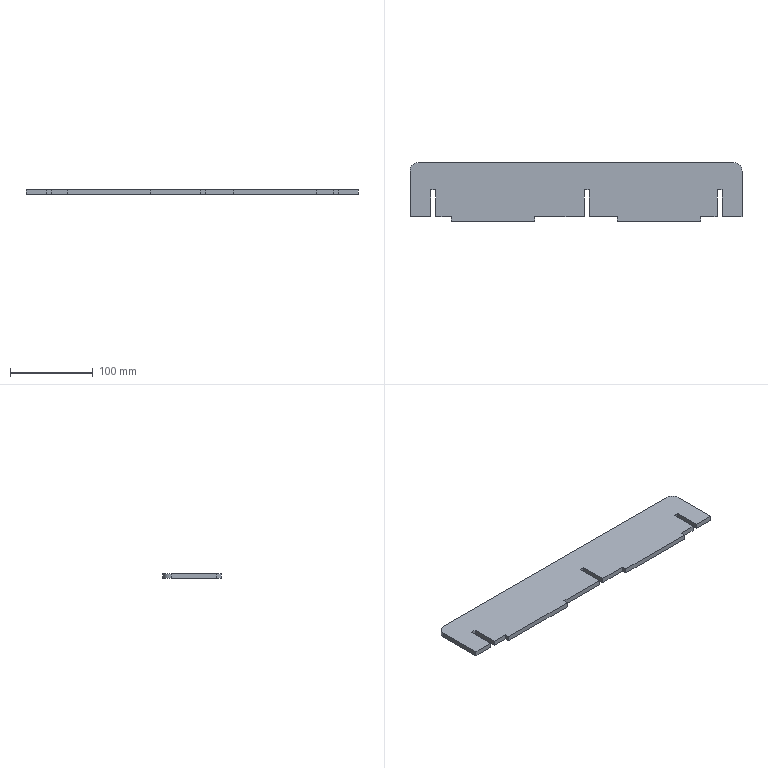Part | SolidWorks | features FlatPattern 1, SMBaseFlange 1, SheetMetal 1 | 1 solid | 28 faces | box 400 x 70.5 x 6 mm | volume 158832 mm3 | plane 26 | cylinder 2 | commonest cylinder face diameters 20 x2
STEP:
#1=CARTESIAN_POINT('',(117.03,-549.5,0.));
#2=VERTEX_POINT('',#1);
#3=CARTESIAN_POINT('',(117.03,-494.5,0.));
#4=VERTEX_POINT('',#3);
#5=CARTESIAN_POINT('',(117.03,-549.5,0.));
#6=DIRECTION('',(0.,1.,0.));
#7=VECTOR('',#6,1000.);
#8=LINE('',#5,#7);
#9=EDGE_CURVE('',#2,#4,#8,.T.);
#10=ORIENTED_EDGE('',*,*,#9,.F.);
#11=CARTESIAN_POINT('',(117.03,-549.5,-6.));
#12=VERTEX_POINT('',#11);
#13=CARTESIAN_POINT('',(117.03,-549.5,-6.));
#14=DIRECTION('',(0.,0.,1.));
#15=VECTOR('',#14,1000.);
#16=LINE('',#13,#15);
#17=EDGE_CURVE('',#12,#2,#16,.T.);
#18=ORIENTED_EDGE('',*,*,#17,.F.);
#19=CARTESIAN_POINT('',(117.03,-494.5,-6.));
#20=VERTEX_POINT('',#19);
#21=CARTESIAN_POINT('',(117.03,-549.5,-6.));
#22=DIRECTION('',(0.,1.,0.));
#23=VECTOR('',#22,1000.);
#24=LINE('',#21,#23);
#25=EDGE_CURVE('',#12,#20,#24,.T.);
#26=ORIENTED_EDGE('',*,*,#25,.T.);
#27=CARTESIAN_POINT('',(117.03,-494.5,-6.));
#28=DIRECTION('',(0.,0.,1.));
#29=VECTOR('',#28,1000.);
#30=LINE('',#27,#29);
#31=EDGE_CURVE('',#20,#4,#30,.T.);
#32=ORIENTED_EDGE('',*,*,#31,.T.);
#33=EDGE_LOOP('',(#10,#18,#26,#32));
#34=FACE_OUTER_BOUND('',#33,.T.);
#35=CARTESIAN_POINT('',(117.03,-549.5,-6.));
#36=DIRECTION('',(1.,0.,0.));
#37=DIRECTION('',(0.,0.,-1.));
#38=AXIS2_PLACEMENT_3D('',#35,#36,#37);
#39=PLANE('',#38);
#40=ADVANCED_FACE('',(#34),#39,.T.);
#41=CARTESIAN_POINT('',(93.03,-549.5,0.));
#42=VERTEX_POINT('',#41);
#43=CARTESIAN_POINT('',(117.03,-549.5,0.));
#44=DIRECTION('',(1.,0.,0.));
#45=VECTOR('',#44,1000.);
#46=LINE('',#43,#45);
#47=EDGE_CURVE('',#42,#2,#46,.T.);
#48=ORIENTED_EDGE('',*,*,#47,.F.);
#49=CARTESIAN_POINT('',(93.03,-549.5,-6.));
#50=VERTEX_POINT('',#49);
#51=CARTESIAN_POINT('',(93.03,-549.5,-6.));
#52=DIRECTION('',(0.,0.,1.));
#53=VECTOR('',#52,1000.);
#54=LINE('',#51,#53);
#55=EDGE_CURVE('',#50,#42,#54,.T.);
#56=ORIENTED_EDGE('',*,*,#55,.F.);
#57=CARTESIAN_POINT('',(117.03,-549.5,-6.));
#58=DIRECTION('',(1.,0.,0.));
#59=VECTOR('',#58,1000.);
#60=LINE('',#57,#59);
#61=EDGE_CURVE('',#50,#12,#60,.T.);
#62=ORIENTED_EDGE('',*,*,#61,.T.);
#63=ORIENTED_EDGE('',*,*,#17,.T.);
#64=EDGE_LOOP('',(#48,#56,#62,#63));
#65=FACE_OUTER_BOUND('',#64,.T.);
#66=CARTESIAN_POINT('',(117.03,-549.5,-6.));
#67=DIRECTION('',(0.,-1.,0.));
#68=DIRECTION('',(1.,0.,0.));
#69=AXIS2_PLACEMENT_3D('',#66,#67,#68);
#70=PLANE('',#69);
#71=ADVANCED_FACE('',(#65),#70,.T.);
#72=CARTESIAN_POINT('',(93.03,-517.,0.));
#73=VERTEX_POINT('',#72);
#74=CARTESIAN_POINT('',(93.03,-549.5,0.));
#75=DIRECTION('',(0.,-1.,0.));
#76=VECTOR('',#75,1000.);
#77=LINE('',#74,#76);
#78=EDGE_CURVE('',#73,#42,#77,.T.);
#79=ORIENTED_EDGE('',*,*,#78,.F.);
#80=CARTESIAN_POINT('',(93.03,-517.,-6.));
#81=VERTEX_POINT('',#80);
#82=CARTESIAN_POINT('',(93.03,-517.,-6.));
#83=DIRECTION('',(0.,0.,1.));
#84=VECTOR('',#83,1000.);
#85=LINE('',#82,#84);
#86=EDGE_CURVE('',#81,#73,#85,.T.);
#87=ORIENTED_EDGE('',*,*,#86,.F.);
#88=CARTESIAN_POINT('',(93.03,-549.5,-6.));
#89=DIRECTION('',(0.,-1.,0.));
#90=VECTOR('',#89,1000.);
#91=LINE('',#88,#90);
#92=EDGE_CURVE('',#81,#50,#91,.T.);
#93=ORIENTED_EDGE('',*,*,#92,.T.);
#94=ORIENTED_EDGE('',*,*,#55,.T.);
#95=EDGE_LOOP('',(#79,#87,#93,#94));
#96=FACE_OUTER_BOUND('',#95,.T.);
#97=CARTESIAN_POINT('',(93.03,-549.5,-6.));
#98=DIRECTION('',(-1.,0.,0.));
#99=DIRECTION('',(0.,-1.,0.));
#100=AXIS2_PLACEMENT_3D('',#97,#98,#99);
#101=PLANE('',#100);
#102=ADVANCED_FACE('',(#96),#101,.T.);
#103=CARTESIAN_POINT('',(87.03,-517.,0.));
#104=VERTEX_POINT('',#103);
#105=CARTESIAN_POINT('',(93.03,-517.,0.));
#106=DIRECTION('',(1.,0.,0.));
#107=VECTOR('',#106,1000.);
#108=LINE('',#105,#107);
#109=EDGE_CURVE('',#104,#73,#108,.T.);
#110=ORIENTED_EDGE('',*,*,#109,.F.);
#111=CARTESIAN_POINT('',(87.03,-517.,-6.));
#112=VERTEX_POINT('',#111);
#113=CARTESIAN_POINT('',(87.03,-517.,-6.));
#114=DIRECTION('',(0.,0.,1.));
#115=VECTOR('',#114,1000.);
#116=LINE('',#113,#115);
#117=EDGE_CURVE('',#112,#104,#116,.T.);
#118=ORIENTED_EDGE('',*,*,#117,.F.);
#119=CARTESIAN_POINT('',(93.03,-517.,-6.));
#120=DIRECTION('',(1.,0.,0.));
#121=VECTOR('',#120,1000.);
#122=LINE('',#119,#121);
#123=EDGE_CURVE('',#112,#81,#122,.T.);
#124=ORIENTED_EDGE('',*,*,#123,.T.);
#125=ORIENTED_EDGE('',*,*,#86,.T.);
#126=EDGE_LOOP('',(#110,#118,#124,#125));
#127=FACE_OUTER_BOUND('',#126,.T.);
#128=CARTESIAN_POINT('',(93.03,-517.,-6.));
#129=DIRECTION('',(0.,-1.,0.));
#130=DIRECTION('',(0.,0.,-1.));
#131=AXIS2_PLACEMENT_3D('',#128,#129,#130);
#132=PLANE('',#131);
#133=ADVANCED_FACE('',(#127),#132,.T.);
#134=CARTESIAN_POINT('',(87.03,-549.5,0.));
#135=VERTEX_POINT('',#134);
#136=CARTESIAN_POINT('',(87.03,-517.,0.));
#137=DIRECTION('',(0.,1.,0.));
#138=VECTOR('',#137,1000.);
#139=LINE('',#136,#138);
#140=EDGE_CURVE('',#135,#104,#139,.T.);
#141=ORIENTED_EDGE('',*,*,#140,.F.);
#142=CARTESIAN_POINT('',(87.03,-549.5,-6.));
#143=VERTEX_POINT('',#142);
#144=CARTESIAN_POINT('',(87.03,-549.5,-6.));
#145=DIRECTION('',(0.,0.,1.));
#146=VECTOR('',#145,1000.);
#147=LINE('',#144,#146);
#148=EDGE_CURVE('',#143,#135,#147,.T.);
#149=ORIENTED_EDGE('',*,*,#148,.F.);
#150=CARTESIAN_POINT('',(87.03,-517.,-6.));
#151=DIRECTION('',(0.,1.,0.));
#152=VECTOR('',#151,1000.);
#153=LINE('',#150,#152);
#154=EDGE_CURVE('',#143,#112,#153,.T.);
#155=ORIENTED_EDGE('',*,*,#154,.T.);
#156=ORIENTED_EDGE('',*,*,#117,.T.);
#157=EDGE_LOOP('',(#141,#149,#155,#156));
#158=FACE_OUTER_BOUND('',#157,.T.);
#159=CARTESIAN_POINT('',(87.03,-517.,-6.));
#160=DIRECTION('',(1.,0.,0.));
#161=DIRECTION('',(0.,0.,-1.));
#162=AXIS2_PLACEMENT_3D('',#159,#160,#161);
#163=PLANE('',#162);
#164=ADVANCED_FACE('',(#158),#163,.T.);
#165=CARTESIAN_POINT('',(67.03,-549.5,0.));
#166=VERTEX_POINT('',#165);
#167=CARTESIAN_POINT('',(87.03,-549.5,0.));
#168=DIRECTION('',(1.,0.,0.));
#169=VECTOR('',#168,1000.);
#170=LINE('',#167,#169);
#171=EDGE_CURVE('',#166,#135,#170,.T.);
#172=ORIENTED_EDGE('',*,*,#171,.F.);
#173=CARTESIAN_POINT('',(67.03,-549.5,-6.));
#174=VERTEX_POINT('',#173);
#175=CARTESIAN_POINT('',(67.03,-549.5,-6.));
#176=DIRECTION('',(0.,0.,1.));
#177=VECTOR('',#176,1000.);
#178=LINE('',#175,#177);
#179=EDGE_CURVE('',#174,#166,#178,.T.);
#180=ORIENTED_EDGE('',*,*,#179,.F.);
#181=CARTESIAN_POINT('',(87.03,-549.5,-6.));
#182=DIRECTION('',(1.,0.,0.));
#183=VECTOR('',#182,1000.);
#184=LINE('',#181,#183);
#185=EDGE_CURVE('',#174,#143,#184,.T.);
#186=ORIENTED_EDGE('',*,*,#185,.T.);
#187=ORIENTED_EDGE('',*,*,#148,.T.);
#188=EDGE_LOOP('',(#172,#180,#186,#187));
#189=FACE_OUTER_BOUND('',#188,.T.);
#190=CARTESIAN_POINT('',(87.03,-549.5,-6.));
#191=DIRECTION('',(0.,-1.,0.));
#192=DIRECTION('',(1.,0.,0.));
#193=AXIS2_PLACEMENT_3D('',#190,#191,#192);
#194=PLANE('',#193);
#195=ADVANCED_FACE('',(#189),#194,.T.);
#196=CARTESIAN_POINT('',(67.03,-555.,0.));
#197=VERTEX_POINT('',#196);
#198=CARTESIAN_POINT('',(67.03,-549.5,0.));
#199=DIRECTION('',(0.,1.,0.));
#200=VECTOR('',#199,1000.);
#201=LINE('',#198,#200);
#202=EDGE_CURVE('',#197,#166,#201,.T.);
#203=ORIENTED_EDGE('',*,*,#202,.F.);
#204=CARTESIAN_POINT('',(67.03,-555.,-6.));
#205=VERTEX_POINT('',#204);
#206=CARTESIAN_POINT('',(67.03,-555.,-6.));
#207=DIRECTION('',(0.,0.,1.));
#208=VECTOR('',#207,1000.);
#209=LINE('',#206,#208);
#210=EDGE_CURVE('',#205,#197,#209,.T.);
#211=ORIENTED_EDGE('',*,*,#210,.F.);
#212=CARTESIAN_POINT('',(67.03,-549.5,-6.));
#213=DIRECTION('',(0.,1.,0.));
#214=VECTOR('',#213,1000.);
#215=LINE('',#212,#214);
#216=EDGE_CURVE('',#205,#174,#215,.T.);
#217=ORIENTED_EDGE('',*,*,#216,.T.);
#218=ORIENTED_EDGE('',*,*,#179,.T.);
#219=EDGE_LOOP('',(#203,#211,#217,#218));
#220=FACE_OUTER_BOUND('',#219,.T.);
#221=CARTESIAN_POINT('',(67.03,-549.5,-6.));
#222=DIRECTION('',(1.,0.,0.));
#223=DIRECTION('',(0.,0.,-1.));
#224=AXIS2_PLACEMENT_3D('',#221,#222,#223);
#225=PLANE('',#224);
#226=ADVANCED_FACE('',(#220),#225,.T.);
#227=CARTESIAN_POINT('',(-32.97,-555.,0.));
#228=VERTEX_POINT('',#227);
#229=CARTESIAN_POINT('',(67.03,-555.,0.));
#230=DIRECTION('',(1.,0.,0.));
#231=VECTOR('',#230,1000.);
#232=LINE('',#229,#231);
#233=EDGE_CURVE('',#228,#197,#232,.T.);
#234=ORIENTED_EDGE('',*,*,#233,.F.);
#235=CARTESIAN_POINT('',(-32.97,-555.,-6.));
#236=VERTEX_POINT('',#235);
#237=CARTESIAN_POINT('',(-32.97,-555.,-6.));
#238=DIRECTION('',(0.,0.,1.));
#239=VECTOR('',#238,1000.);
#240=LINE('',#237,#239);
#241=EDGE_CURVE('',#236,#228,#240,.T.);
#242=ORIENTED_EDGE('',*,*,#241,.F.);
#243=CARTESIAN_POINT('',(67.03,-555.,-6.));
#244=DIRECTION('',(1.,0.,0.));
#245=VECTOR('',#244,1000.);
#246=LINE('',#243,#245);
#247=EDGE_CURVE('',#236,#205,#246,.T.);
#248=ORIENTED_EDGE('',*,*,#247,.T.);
#249=ORIENTED_EDGE('',*,*,#210,.T.);
#250=EDGE_LOOP('',(#234,#242,#248,#249));
#251=FACE_OUTER_BOUND('',#250,.T.);
#252=CARTESIAN_POINT('',(67.03,-555.,-6.));
#253=DIRECTION('',(0.,-1.,0.));
#254=DIRECTION('',(0.,0.,-1.));
#255=AXIS2_PLACEMENT_3D('',#252,#253,#254);
#256=PLANE('',#255);
#257=ADVANCED_FACE('',(#251),#256,.T.);
#258=CARTESIAN_POINT('',(-32.97,-549.5,0.));
#259=VERTEX_POINT('',#258);
#260=CARTESIAN_POINT('',(-32.97,-555.,0.));
#261=DIRECTION('',(0.,-1.,0.));
#262=VECTOR('',#261,1000.);
#263=LINE('',#260,#262);
#264=EDGE_CURVE('',#259,#228,#263,.T.);
#265=ORIENTED_EDGE('',*,*,#264,.F.);
#266=CARTESIAN_POINT('',(-32.97,-549.5,-6.));
#267=VERTEX_POINT('',#266);
#268=CARTESIAN_POINT('',(-32.97,-549.5,-6.));
#269=DIRECTION('',(0.,0.,1.));
#270=VECTOR('',#269,1000.);
#271=LINE('',#268,#270);
#272=EDGE_CURVE('',#267,#259,#271,.T.);
#273=ORIENTED_EDGE('',*,*,#272,.F.);
#274=CARTESIAN_POINT('',(-32.97,-555.,-6.));
#275=DIRECTION('',(0.,-1.,0.));
#276=VECTOR('',#275,1000.);
#277=LINE('',#274,#276);
#278=EDGE_CURVE('',#267,#236,#277,.T.);
#279=ORIENTED_EDGE('',*,*,#278,.T.);
#280=ORIENTED_EDGE('',*,*,#241,.T.);
#281=EDGE_LOOP('',(#265,#273,#279,#280));
#282=FACE_OUTER_BOUND('',#281,.T.);
#283=CARTESIAN_POINT('',(-32.97,-555.,-6.));
#284=DIRECTION('',(-1.,0.,0.));
#285=DIRECTION('',(0.,0.,1.));
#286=AXIS2_PLACEMENT_3D('',#283,#284,#285);
#287=PLANE('',#286);
#288=ADVANCED_FACE('',(#282),#287,.T.);
#289=CARTESIAN_POINT('',(-66.97,-549.5,0.));
#290=VERTEX_POINT('',#289);
#291=CARTESIAN_POINT('',(-32.97,-549.5,0.));
#292=DIRECTION('',(1.,0.,0.));
#293=VECTOR('',#292,1000.);
#294=LINE('',#291,#293);
#295=EDGE_CURVE('',#290,#259,#294,.T.);
#296=ORIENTED_EDGE('',*,*,#295,.F.);
#297=CARTESIAN_POINT('',(-66.97,-549.5,-6.));
#298=VERTEX_POINT('',#297);
#299=CARTESIAN_POINT('',(-66.97,-549.5,-6.));
#300=DIRECTION('',(0.,0.,1.));
#301=VECTOR('',#300,1000.);
#302=LINE('',#299,#301);
#303=EDGE_CURVE('',#298,#290,#302,.T.);
#304=ORIENTED_EDGE('',*,*,#303,.F.);
#305=CARTESIAN_POINT('',(-32.97,-549.5,-6.));
#306=DIRECTION('',(1.,0.,0.));
#307=VECTOR('',#306,1000.);
#308=LINE('',#305,#307);
#309=EDGE_CURVE('',#298,#267,#308,.T.);
#310=ORIENTED_EDGE('',*,*,#309,.T.);
#311=ORIENTED_EDGE('',*,*,#272,.T.);
#312=EDGE_LOOP('',(#296,#304,#310,#311));
#313=FACE_OUTER_BOUND('',#312,.T.);
#314=CARTESIAN_POINT('',(-32.97,-549.5,-6.));
#315=DIRECTION('',(0.,-1.,0.));
#316=DIRECTION('',(1.,0.,0.));
#317=AXIS2_PLACEMENT_3D('',#314,#315,#316);
#318=PLANE('',#317);
#319=ADVANCED_FACE('',(#313),#318,.T.);
#320=CARTESIAN_POINT('',(-66.97,-517.,0.));
#321=VERTEX_POINT('',#320);
#322=CARTESIAN_POINT('',(-66.97,-549.5,0.));
#323=DIRECTION('',(0.,-1.,0.));
#324=VECTOR('',#323,1000.);
#325=LINE('',#322,#324);
#326=EDGE_CURVE('',#321,#290,#325,.T.);
#327=ORIENTED_EDGE('',*,*,#326,.F.);
#328=CARTESIAN_POINT('',(-66.97,-517.,-6.));
#329=VERTEX_POINT('',#328);
#330=CARTESIAN_POINT('',(-66.97,-517.,-6.));
#331=DIRECTION('',(0.,0.,1.));
#332=VECTOR('',#331,1000.);
#333=LINE('',#330,#332);
#334=EDGE_CURVE('',#329,#321,#333,.T.);
#335=ORIENTED_EDGE('',*,*,#334,.F.);
#336=CARTESIAN_POINT('',(-66.97,-549.5,-6.));
#337=DIRECTION('',(0.,-1.,0.));
#338=VECTOR('',#337,1000.);
#339=LINE('',#336,#338);
#340=EDGE_CURVE('',#329,#298,#339,.T.);
#341=ORIENTED_EDGE('',*,*,#340,.T.);
#342=ORIENTED_EDGE('',*,*,#303,.T.);
#343=EDGE_LOOP('',(#327,#335,#341,#342));
#344=FACE_OUTER_BOUND('',#343,.T.);
#345=CARTESIAN_POINT('',(-66.97,-549.5,-6.));
#346=DIRECTION('',(-1.,0.,0.));
#347=DIRECTION('',(0.,0.,1.));
#348=AXIS2_PLACEMENT_3D('',#345,#346,#347);
#349=PLANE('',#348);
#350=ADVANCED_FACE('',(#344),#349,.T.);
#351=CARTESIAN_POINT('',(-72.97,-517.,0.));
#352=VERTEX_POINT('',#351);
#353=CARTESIAN_POINT('',(-66.97,-517.,0.));
#354=DIRECTION('',(1.,0.,0.));
#355=VECTOR('',#354,1000.);
#356=LINE('',#353,#355);
#357=EDGE_CURVE('',#352,#321,#356,.T.);
#358=ORIENTED_EDGE('',*,*,#357,.F.);
#359=CARTESIAN_POINT('',(-72.97,-517.,-6.));
#360=VERTEX_POINT('',#359);
#361=CARTESIAN_POINT('',(-72.97,-517.,-6.));
#362=DIRECTION('',(0.,0.,1.));
#363=VECTOR('',#362,1000.);
#364=LINE('',#361,#363);
#365=EDGE_CURVE('',#360,#352,#364,.T.);
#366=ORIENTED_EDGE('',*,*,#365,.F.);
#367=CARTESIAN_POINT('',(-66.97,-517.,-6.));
#368=DIRECTION('',(1.,0.,0.));
#369=VECTOR('',#368,1000.);
#370=LINE('',#367,#369);
#371=EDGE_CURVE('',#360,#329,#370,.T.);
#372=ORIENTED_EDGE('',*,*,#371,.T.);
#373=ORIENTED_EDGE('',*,*,#334,.T.);
#374=EDGE_LOOP('',(#358,#366,#372,#373));
#375=FACE_OUTER_BOUND('',#374,.T.);
#376=CARTESIAN_POINT('',(-66.97,-517.,-6.));
#377=DIRECTION('',(0.,-1.,0.));
#378=DIRECTION('',(0.,0.,-1.));
#379=AXIS2_PLACEMENT_3D('',#376,#377,#378);
#380=PLANE('',#379);
#381=ADVANCED_FACE('',(#375),#380,.T.);
#382=CARTESIAN_POINT('',(-72.97,-549.5,0.));
#383=VERTEX_POINT('',#382);
#384=CARTESIAN_POINT('',(-72.97,-517.,0.));
#385=DIRECTION('',(0.,1.,0.));
#386=VECTOR('',#385,1000.);
#387=LINE('',#384,#386);
#388=EDGE_CURVE('',#383,#352,#387,.T.);
#389=ORIENTED_EDGE('',*,*,#388,.F.);
#390=CARTESIAN_POINT('',(-72.97,-549.5,-6.));
#391=VERTEX_POINT('',#390);
#392=CARTESIAN_POINT('',(-72.97,-549.5,-6.));
#393=DIRECTION('',(0.,0.,1.));
#394=VECTOR('',#393,1000.);
#395=LINE('',#392,#394);
#396=EDGE_CURVE('',#391,#383,#395,.T.);
#397=ORIENTED_EDGE('',*,*,#396,.F.);
#398=CARTESIAN_POINT('',(-72.97,-517.,-6.));
#399=DIRECTION('',(0.,1.,0.));
#400=VECTOR('',#399,1000.);
#401=LINE('',#398,#400);
#402=EDGE_CURVE('',#391,#360,#401,.T.);
#403=ORIENTED_EDGE('',*,*,#402,.T.);
#404=ORIENTED_EDGE('',*,*,#365,.T.);
#405=EDGE_LOOP('',(#389,#397,#403,#404));
#406=FACE_OUTER_BOUND('',#405,.T.);
#407=CARTESIAN_POINT('',(-72.97,-517.,-6.));
#408=DIRECTION('',(1.,0.,0.));
#409=DIRECTION('',(0.,0.,-1.));
#410=AXIS2_PLACEMENT_3D('',#407,#408,#409);
#411=PLANE('',#410);
#412=ADVANCED_FACE('',(#406),#411,.T.);
#413=CARTESIAN_POINT('',(-132.97,-549.5,0.));
#414=VERTEX_POINT('',#413);
#415=CARTESIAN_POINT('',(-72.97,-549.5,0.));
#416=DIRECTION('',(1.,0.,0.));
#417=VECTOR('',#416,1000.);
#418=LINE('',#415,#417);
#419=EDGE_CURVE('',#414,#383,#418,.T.);
#420=ORIENTED_EDGE('',*,*,#419,.F.);
#421=CARTESIAN_POINT('',(-132.97,-549.5,-6.));
#422=VERTEX_POINT('',#421);
#423=CARTESIAN_POINT('',(-132.97,-549.5,-6.));
#424=DIRECTION('',(0.,0.,1.));
#425=VECTOR('',#424,1000.);
#426=LINE('',#423,#425);
#427=EDGE_CURVE('',#422,#414,#426,.T.);
#428=ORIENTED_EDGE('',*,*,#427,.F.);
#429=CARTESIAN_POINT('',(-72.97,-549.5,-6.));
#430=DIRECTION('',(1.,0.,0.));
#431=VECTOR('',#430,1000.);
#432=LINE('',#429,#431);
#433=EDGE_CURVE('',#422,#391,#432,.T.);
#434=ORIENTED_EDGE('',*,*,#433,.T.);
#435=ORIENTED_EDGE('',*,*,#396,.T.);
#436=EDGE_LOOP('',(#420,#428,#434,#435));
#437=FACE_OUTER_BOUND('',#436,.T.);
#438=CARTESIAN_POINT('',(-72.97,-549.5,-6.));
#439=DIRECTION('',(0.,-1.,0.));
#440=DIRECTION('',(1.,0.,0.));
#441=AXIS2_PLACEMENT_3D('',#438,#439,#440);
#442=PLANE('',#441);
#443=ADVANCED_FACE('',(#437),#442,.T.);
#444=CARTESIAN_POINT('',(-132.97,-555.,0.));
#445=VERTEX_POINT('',#444);
#446=CARTESIAN_POINT('',(-132.97,-555.,0.));
#447=DIRECTION('',(0.,1.,0.));
#448=VECTOR('',#447,1000.);
#449=LINE('',#446,#448);
#450=EDGE_CURVE('',#445,#414,#449,.T.);
#451=ORIENTED_EDGE('',*,*,#450,.F.);
#452=CARTESIAN_POINT('',(-132.97,-555.,-6.));
#453=VERTEX_POINT('',#452);
#454=CARTESIAN_POINT('',(-132.97,-555.,-6.));
#455=DIRECTION('',(0.,0.,1.));
#456=VECTOR('',#455,1000.);
#457=LINE('',#454,#456);
#458=EDGE_CURVE('',#453,#445,#457,.T.);
#459=ORIENTED_EDGE('',*,*,#458,.F.);
#460=CARTESIAN_POINT('',(-132.97,-555.,-6.));
#461=DIRECTION('',(0.,1.,0.));
#462=VECTOR('',#461,1000.);
#463=LINE('',#460,#462);
#464=EDGE_CURVE('',#453,#422,#463,.T.);
#465=ORIENTED_EDGE('',*,*,#464,.T.);
#466=ORIENTED_EDGE('',*,*,#427,.T.);
#467=EDGE_LOOP('',(#451,#459,#465,#466));
#468=FACE_OUTER_BOUND('',#467,.T.);
#469=CARTESIAN_POINT('',(-132.97,-555.,-6.));
#470=DIRECTION('',(1.,0.,0.));
#471=DIRECTION('',(0.,0.,-1.));
#472=AXIS2_PLACEMENT_3D('',#469,#470,#471);
#473=PLANE('',#472);
#474=ADVANCED_FACE('',(#468),#473,.T.);
#475=CARTESIAN_POINT('',(-232.97,-555.,0.));
#476=VERTEX_POINT('',#475);
#477=CARTESIAN_POINT('',(-232.97,-555.,0.));
#478=DIRECTION('',(1.,0.,0.));
#479=VECTOR('',#478,1000.);
#480=LINE('',#477,#479);
#481=EDGE_CURVE('',#476,#445,#480,.T.);
#482=ORIENTED_EDGE('',*,*,#481,.F.);
#483=CARTESIAN_POINT('',(-232.97,-555.,-6.));
#484=VERTEX_POINT('',#483);
#485=CARTESIAN_POINT('',(-232.97,-555.,-6.));
#486=DIRECTION('',(0.,0.,1.));
#487=VECTOR('',#486,1000.);
#488=LINE('',#485,#487);
#489=EDGE_CURVE('',#484,#476,#488,.T.);
#490=ORIENTED_EDGE('',*,*,#489,.F.);
#491=CARTESIAN_POINT('',(-232.97,-555.,-6.));
#492=DIRECTION('',(1.,0.,0.));
#493=VECTOR('',#492,1000.);
#494=LINE('',#491,#493);
#495=EDGE_CURVE('',#484,#453,#494,.T.);
#496=ORIENTED_EDGE('',*,*,#495,.T.);
#497=ORIENTED_EDGE('',*,*,#458,.T.);
#498=EDGE_LOOP('',(#482,#490,#496,#497));
#499=FACE_OUTER_BOUND('',#498,.T.);
#500=CARTESIAN_POINT('',(-232.97,-555.,-6.));
#501=DIRECTION('',(0.,-1.,0.));
#502=DIRECTION('',(0.,0.,-1.));
#503=AXIS2_PLACEMENT_3D('',#500,#501,#502);
#504=PLANE('',#503);
#505=ADVANCED_FACE('',(#499),#504,.T.);
#506=CARTESIAN_POINT('',(-232.97,-549.5,0.));
#507=VERTEX_POINT('',#506);
#508=CARTESIAN_POINT('',(-232.97,-549.5,0.));
#509=DIRECTION('',(0.,-1.,0.));
#510=VECTOR('',#509,1000.);
#511=LINE('',#508,#510);
#512=EDGE_CURVE('',#507,#476,#511,.T.);
#513=ORIENTED_EDGE('',*,*,#512,.F.);
#514=CARTESIAN_POINT('',(-232.97,-549.5,-6.));
#515=VERTEX_POINT('',#514);
#516=CARTESIAN_POINT('',(-232.97,-549.5,-6.));
#517=DIRECTION('',(0.,0.,1.));
#518=VECTOR('',#517,1000.);
#519=LINE('',#516,#518);
#520=EDGE_CURVE('',#515,#507,#519,.T.);
#521=ORIENTED_EDGE('',*,*,#520,.F.);
#522=CARTESIAN_POINT('',(-232.97,-549.5,-6.));
#523=DIRECTION('',(0.,-1.,0.));
#524=VECTOR('',#523,1000.);
#525=LINE('',#522,#524);
#526=EDGE_CURVE('',#515,#484,#525,.T.);
#527=ORIENTED_EDGE('',*,*,#526,.T.);
#528=ORIENTED_EDGE('',*,*,#489,.T.);
#529=EDGE_LOOP('',(#513,#521,#527,#528));
#530=FACE_OUTER_BOUND('',#529,.T.);
#531=CARTESIAN_POINT('',(-232.97,-549.5,-6.));
#532=DIRECTION('',(-1.,0.,0.));
#533=DIRECTION('',(0.,0.,1.));
#534=AXIS2_PLACEMENT_3D('',#531,#532,#533);
#535=PLANE('',#534);
#536=ADVANCED_FACE('',(#530),#535,.T.);
#537=CARTESIAN_POINT('',(-251.97,-549.5,0.));
#538=VERTEX_POINT('',#537);
#539=CARTESIAN_POINT('',(-232.97,-549.5,0.));
#540=DIRECTION('',(1.,0.,0.));
#541=VECTOR('',#540,1000.);
#542=LINE('',#539,#541);
#543=EDGE_CURVE('',#538,#507,#542,.T.);
#544=ORIENTED_EDGE('',*,*,#543,.F.);
#545=CARTESIAN_POINT('',(-251.97,-549.5,-6.));
#546=VERTEX_POINT('',#545);
#547=CARTESIAN_POINT('',(-251.97,-549.5,-6.));
#548=DIRECTION('',(0.,0.,1.));
#549=VECTOR('',#548,1000.);
#550=LINE('',#547,#549);
#551=EDGE_CURVE('',#546,#538,#550,.T.);
#552=ORIENTED_EDGE('',*,*,#551,.F.);
#553=CARTESIAN_POINT('',(-232.97,-549.5,-6.));
#554=DIRECTION('',(1.,0.,0.));
#555=VECTOR('',#554,1000.);
#556=LINE('',#553,#555);
#557=EDGE_CURVE('',#546,#515,#556,.T.);
#558=ORIENTED_EDGE('',*,*,#557,.T.);
#559=ORIENTED_EDGE('',*,*,#520,.T.);
#560=EDGE_LOOP('',(#544,#552,#558,#559));
#561=FACE_OUTER_BOUND('',#560,.T.);
#562=CARTESIAN_POINT('',(-232.97,-549.5,-6.));
#563=DIRECTION('',(0.,-1.,0.));
#564=DIRECTION('',(1.,0.,0.));
#565=AXIS2_PLACEMENT_3D('',#562,#563,#564);
#566=PLANE('',#565);
#567=ADVANCED_FACE('',(#561),#566,.T.);
#568=CARTESIAN_POINT('',(-251.97,-517.,0.));
#569=VERTEX_POINT('',#568);
#570=CARTESIAN_POINT('',(-251.97,-549.5,0.));
#571=DIRECTION('',(0.,-1.,0.));
#572=VECTOR('',#571,1000.);
#573=LINE('',#570,#572);
#574=EDGE_CURVE('',#569,#538,#573,.T.);
#575=ORIENTED_EDGE('',*,*,#574,.F.);
#576=CARTESIAN_POINT('',(-251.97,-517.,-6.));
#577=VERTEX_POINT('',#576);
#578=CARTESIAN_POINT('',(-251.97,-517.,-6.));
#579=DIRECTION('',(0.,0.,1.));
#580=VECTOR('',#579,1000.);
#581=LINE('',#578,#580);
#582=EDGE_CURVE('',#577,#569,#581,.T.);
#583=ORIENTED_EDGE('',*,*,#582,.F.);
#584=CARTESIAN_POINT('',(-251.97,-549.5,-6.));
#585=DIRECTION('',(0.,-1.,0.));
#586=VECTOR('',#585,1000.);
#587=LINE('',#584,#586);
#588=EDGE_CURVE('',#577,#546,#587,.T.);
#589=ORIENTED_EDGE('',*,*,#588,.T.);
#590=ORIENTED_EDGE('',*,*,#551,.T.);
#591=EDGE_LOOP('',(#575,#583,#589,#590));
#592=FACE_OUTER_BOUND('',#591,.T.);
#593=CARTESIAN_POINT('',(-251.97,-549.5,-6.));
#594=DIRECTION('',(-1.,0.,0.));
#595=DIRECTION('',(0.,-1.,0.));
#596=AXIS2_PLACEMENT_3D('',#593,#594,#595);
#597=PLANE('',#596);
#598=ADVANCED_FACE('',(#592),#597,.T.);
#599=CARTESIAN_POINT('',(-257.97,-517.,0.));
#600=VERTEX_POINT('',#599);
#601=CARTESIAN_POINT('',(-251.97,-517.,0.));
#602=DIRECTION('',(1.,0.,0.));
#603=VECTOR('',#602,1000.);
#604=LINE('',#601,#603);
#605=EDGE_CURVE('',#600,#569,#604,.T.);
#606=ORIENTED_EDGE('',*,*,#605,.F.);
#607=CARTESIAN_POINT('',(-257.97,-517.,-6.));
#608=VERTEX_POINT('',#607);
#609=CARTESIAN_POINT('',(-257.97,-517.,-6.));
#610=DIRECTION('',(0.,0.,1.));
#611=VECTOR('',#610,1000.);
#612=LINE('',#609,#611);
#613=EDGE_CURVE('',#608,#600,#612,.T.);
#614=ORIENTED_EDGE('',*,*,#613,.F.);
#615=CARTESIAN_POINT('',(-251.97,-517.,-6.));
#616=DIRECTION('',(1.,0.,0.));
#617=VECTOR('',#616,1000.);
#618=LINE('',#615,#617);
#619=EDGE_CURVE('',#608,#577,#618,.T.);
#620=ORIENTED_EDGE('',*,*,#619,.T.);
#621=ORIENTED_EDGE('',*,*,#582,.T.);
#622=EDGE_LOOP('',(#606,#614,#620,#621));
#623=FACE_OUTER_BOUND('',#622,.T.);
#624=CARTESIAN_POINT('',(-251.97,-517.,-6.));
#625=DIRECTION('',(0.,-1.,0.));
#626=DIRECTION('',(0.,0.,-1.));
#627=AXIS2_PLACEMENT_3D('',#624,#625,#626);
#628=PLANE('',#627);
#629=ADVANCED_FACE('',(#623),#628,.T.);
#630=CARTESIAN_POINT('',(-257.97,-549.5,0.));
#631=VERTEX_POINT('',#630);
#632=CARTESIAN_POINT('',(-257.97,-517.,0.));
#633=DIRECTION('',(0.,1.,0.));
#634=VECTOR('',#633,1000.);
#635=LINE('',#632,#634);
#636=EDGE_CURVE('',#631,#600,#635,.T.);
#637=ORIENTED_EDGE('',*,*,#636,.F.);
#638=CARTESIAN_POINT('',(-257.97,-549.5,-6.));
#639=VERTEX_POINT('',#638);
#640=CARTESIAN_POINT('',(-257.97,-549.5,-6.));
#641=DIRECTION('',(0.,0.,1.));
#642=VECTOR('',#641,1000.);
#643=LINE('',#640,#642);
#644=EDGE_CURVE('',#639,#631,#643,.T.);
#645=ORIENTED_EDGE('',*,*,#644,.F.);
#646=CARTESIAN_POINT('',(-257.97,-517.,-6.));
#647=DIRECTION('',(0.,1.,0.));
#648=VECTOR('',#647,1000.);
#649=LINE('',#646,#648);
#650=EDGE_CURVE('',#639,#608,#649,.T.);
#651=ORIENTED_EDGE('',*,*,#650,.T.);
#652=ORIENTED_EDGE('',*,*,#613,.T.);
#653=EDGE_LOOP('',(#637,#645,#651,#652));
#654=FACE_OUTER_BOUND('',#653,.T.);
#655=CARTESIAN_POINT('',(-257.97,-517.,-6.));
#656=DIRECTION('',(1.,0.,0.));
#657=DIRECTION('',(0.,0.,-1.));
#658=AXIS2_PLACEMENT_3D('',#655,#656,#657);
#659=PLANE('',#658);
#660=ADVANCED_FACE('',(#654),#659,.T.);
#661=CARTESIAN_POINT('',(-282.97,-549.5,0.));
#662=VERTEX_POINT('',#661);
#663=CARTESIAN_POINT('',(-257.97,-549.5,0.));
#664=DIRECTION('',(1.,0.,0.));
#665=VECTOR('',#664,1000.);
#666=LINE('',#663,#665);
#667=EDGE_CURVE('',#662,#631,#666,.T.);
#668=ORIENTED_EDGE('',*,*,#667,.F.);
#669=CARTESIAN_POINT('',(-282.97,-549.5,-6.));
#670=VERTEX_POINT('',#669);
#671=CARTESIAN_POINT('',(-282.97,-549.5,-6.));
#672=DIRECTION('',(0.,0.,1.));
#673=VECTOR('',#672,1000.);
#674=LINE('',#671,#673);
#675=EDGE_CURVE('',#670,#662,#674,.T.);
#676=ORIENTED_EDGE('',*,*,#675,.F.);
#677=CARTESIAN_POINT('',(-257.97,-549.5,-6.));
#678=DIRECTION('',(1.,0.,0.));
#679=VECTOR('',#678,1000.);
#680=LINE('',#677,#679);
#681=EDGE_CURVE('',#670,#639,#680,.T.);
#682=ORIENTED_EDGE('',*,*,#681,.T.);
#683=ORIENTED_EDGE('',*,*,#644,.T.);
#684=EDGE_LOOP('',(#668,#676,#682,#683));
#685=FACE_OUTER_BOUND('',#684,.T.);
#686=CARTESIAN_POINT('',(-257.97,-549.5,-6.));
#687=DIRECTION('',(0.,-1.,0.));
#688=DIRECTION('',(1.,0.,0.));
#689=AXIS2_PLACEMENT_3D('',#686,#687,#688);
#690=PLANE('',#689);
#691=ADVANCED_FACE('',(#685),#690,.T.);
#692=CARTESIAN_POINT('',(-282.97,-494.5,0.));
#693=VERTEX_POINT('',#692);
#694=CARTESIAN_POINT('',(-282.97,-549.5,0.));
#695=DIRECTION('',(0.,-1.,0.));
#696=VECTOR('',#695,1000.);
#697=LINE('',#694,#696);
#698=EDGE_CURVE('',#693,#662,#697,.T.);
#699=ORIENTED_EDGE('',*,*,#698,.F.);
#700=CARTESIAN_POINT('',(-282.97,-494.5,-6.));
#701=VERTEX_POINT('',#700);
#702=CARTESIAN_POINT('',(-282.97,-494.5,-6.));
#703=DIRECTION('',(0.,0.,1.));
#704=VECTOR('',#703,1000.);
#705=LINE('',#702,#704);
#706=EDGE_CURVE('',#701,#693,#705,.T.);
#707=ORIENTED_EDGE('',*,*,#706,.F.);
#708=CARTESIAN_POINT('',(-282.97,-549.5,-6.));
#709=DIRECTION('',(0.,-1.,0.));
#710=VECTOR('',#709,1000.);
#711=LINE('',#708,#710);
#712=EDGE_CURVE('',#701,#670,#711,.T.);
#713=ORIENTED_EDGE('',*,*,#712,.T.);
#714=ORIENTED_EDGE('',*,*,#675,.T.);
#715=EDGE_LOOP('',(#699,#707,#713,#714));
#716=FACE_OUTER_BOUND('',#715,.T.);
#717=CARTESIAN_POINT('',(-282.97,-549.5,-6.));
#718=DIRECTION('',(-1.,0.,0.));
#719=DIRECTION('',(0.,-1.,0.));
#720=AXIS2_PLACEMENT_3D('',#717,#718,#719);
#721=PLANE('',#720);
#722=ADVANCED_FACE('',(#716),#721,.T.);
#723=CARTESIAN_POINT('',(-272.97,-484.5,0.));
#724=VERTEX_POINT('',#723);
#725=CARTESIAN_POINT('',(-272.97,-494.5,0.));
#726=DIRECTION('',(0.,0.,1.));
#727=DIRECTION('',(1.,0.,0.));
#728=AXIS2_PLACEMENT_3D('',#725,#726,#727);
#729=CIRCLE('',#728,10.);
#730=EDGE_CURVE('',#724,#693,#729,.T.);
#731=ORIENTED_EDGE('',*,*,#730,.F.);
#732=CARTESIAN_POINT('',(-272.97,-484.5,-6.));
#733=VERTEX_POINT('',#732);
#734=CARTESIAN_POINT('',(-272.97,-484.5,-6.));
#735=DIRECTION('',(0.,0.,1.));
#736=VECTOR('',#735,1000.);
#737=LINE('',#734,#736);
#738=EDGE_CURVE('',#733,#724,#737,.T.);
#739=ORIENTED_EDGE('',*,*,#738,.F.);
#740=CARTESIAN_POINT('',(-272.97,-494.5,-6.));
#741=DIRECTION('',(0.,0.,1.));
#742=DIRECTION('',(1.,0.,0.));
#743=AXIS2_PLACEMENT_3D('',#740,#741,#742);
#744=CIRCLE('',#743,10.);
#745=EDGE_CURVE('',#733,#701,#744,.T.);
#746=ORIENTED_EDGE('',*,*,#745,.T.);
#747=ORIENTED_EDGE('',*,*,#706,.T.);
#748=EDGE_LOOP('',(#731,#739,#746,#747));
#749=FACE_OUTER_BOUND('',#748,.T.);
#750=CARTESIAN_POINT('',(-272.97,-494.5,-6.));
#751=DIRECTION('',(0.,0.,1.));
#752=DIRECTION('',(1.,0.,0.));
#753=AXIS2_PLACEMENT_3D('',#750,#751,#752);
#754=CYLINDRICAL_SURFACE('',#753,10.);
#755=ADVANCED_FACE('',(#749),#754,.T.);
#756=CARTESIAN_POINT('',(107.03,-484.5,0.));
#757=VERTEX_POINT('',#756);
#758=CARTESIAN_POINT('',(107.03,-484.5,0.));
#759=DIRECTION('',(-1.,0.,0.));
#760=VECTOR('',#759,1000.);
#761=LINE('',#758,#760);
#762=EDGE_CURVE('',#757,#724,#761,.T.);
#763=ORIENTED_EDGE('',*,*,#762,.F.);
#764=CARTESIAN_POINT('',(107.03,-484.5,-6.));
#765=VERTEX_POINT('',#764);
#766=CARTESIAN_POINT('',(107.03,-484.5,-6.));
#767=DIRECTION('',(0.,0.,1.));
#768=VECTOR('',#767,1000.);
#769=LINE('',#766,#768);
#770=EDGE_CURVE('',#765,#757,#769,.T.);
#771=ORIENTED_EDGE('',*,*,#770,.F.);
#772=CARTESIAN_POINT('',(107.03,-484.5,-6.));
#773=DIRECTION('',(-1.,0.,0.));
#774=VECTOR('',#773,1000.);
#775=LINE('',#772,#774);
#776=EDGE_CURVE('',#765,#733,#775,.T.);
#777=ORIENTED_EDGE('',*,*,#776,.T.);
#778=ORIENTED_EDGE('',*,*,#738,.T.);
#779=EDGE_LOOP('',(#763,#771,#777,#778));
#780=FACE_OUTER_BOUND('',#779,.T.);
#781=CARTESIAN_POINT('',(107.03,-484.5,-6.));
#782=DIRECTION('',(0.,1.,0.));
#783=DIRECTION('',(-1.,0.,0.));
#784=AXIS2_PLACEMENT_3D('',#781,#782,#783);
#785=PLANE('',#784);
#786=ADVANCED_FACE('',(#780),#785,.T.);
#787=CARTESIAN_POINT('',(107.03,-494.5,0.));
#788=DIRECTION('',(0.,0.,1.));
#789=DIRECTION('',(1.,0.,0.));
#790=AXIS2_PLACEMENT_3D('',#787,#788,#789);
#791=CIRCLE('',#790,10.);
#792=EDGE_CURVE('',#4,#757,#791,.T.);
#793=ORIENTED_EDGE('',*,*,#792,.F.);
#794=ORIENTED_EDGE('',*,*,#31,.F.);
#795=CARTESIAN_POINT('',(107.03,-494.5,-6.));
#796=DIRECTION('',(0.,0.,1.));
#797=DIRECTION('',(1.,0.,0.));
#798=AXIS2_PLACEMENT_3D('',#795,#796,#797);
#799=CIRCLE('',#798,10.);
#800=EDGE_CURVE('',#20,#765,#799,.T.);
#801=ORIENTED_EDGE('',*,*,#800,.T.);
#802=ORIENTED_EDGE('',*,*,#770,.T.);
#803=EDGE_LOOP('',(#793,#794,#801,#802));
#804=FACE_OUTER_BOUND('',#803,.T.);
#805=CARTESIAN_POINT('',(107.03,-494.5,-6.));
#806=DIRECTION('',(0.,0.,1.));
#807=DIRECTION('',(1.,0.,0.));
#808=AXIS2_PLACEMENT_3D('',#805,#806,#807);
#809=CYLINDRICAL_SURFACE('',#808,10.);
#810=ADVANCED_FACE('',(#804),#809,.T.);
#811=ORIENTED_EDGE('',*,*,#25,.F.);
#812=ORIENTED_EDGE('',*,*,#61,.F.);
#813=ORIENTED_EDGE('',*,*,#92,.F.);
#814=ORIENTED_EDGE('',*,*,#123,.F.);
#815=ORIENTED_EDGE('',*,*,#154,.F.);
#816=ORIENTED_EDGE('',*,*,#185,.F.);
#817=ORIENTED_EDGE('',*,*,#216,.F.);
#818=ORIENTED_EDGE('',*,*,#247,.F.);
#819=ORIENTED_EDGE('',*,*,#278,.F.);
#820=ORIENTED_EDGE('',*,*,#309,.F.);
#821=ORIENTED_EDGE('',*,*,#340,.F.);
#822=ORIENTED_EDGE('',*,*,#371,.F.);
#823=ORIENTED_EDGE('',*,*,#402,.F.);
#824=ORIENTED_EDGE('',*,*,#433,.F.);
#825=ORIENTED_EDGE('',*,*,#464,.F.);
#826=ORIENTED_EDGE('',*,*,#495,.F.);
#827=ORIENTED_EDGE('',*,*,#526,.F.);
#828=ORIENTED_EDGE('',*,*,#557,.F.);
#829=ORIENTED_EDGE('',*,*,#588,.F.);
#830=ORIENTED_EDGE('',*,*,#619,.F.);
#831=ORIENTED_EDGE('',*,*,#650,.F.);
#832=ORIENTED_EDGE('',*,*,#681,.F.);
#833=ORIENTED_EDGE('',*,*,#712,.F.);
#834=ORIENTED_EDGE('',*,*,#745,.F.);
#835=ORIENTED_EDGE('',*,*,#776,.F.);
#836=ORIENTED_EDGE('',*,*,#800,.F.);
#837=EDGE_LOOP('',(#811,#812,#813,#814,#815,#816,#817,#818,#819,#820,#821,#822,#823,#824,#825,#826,#827,#828,#829,#830,#831,#832,#833,#834,#835,#836));
#838=FACE_OUTER_BOUND('',#837,.T.);
#839=CARTESIAN_POINT('',(107.03,-494.5,-6.));
#840=DIRECTION('',(0.,0.,1.));
#841=DIRECTION('',(1.,0.,0.));
#842=AXIS2_PLACEMENT_3D('',#839,#840,#841);
#843=PLANE('',#842);
#844=ADVANCED_FACE('',(#838),#843,.F.);
#845=ORIENTED_EDGE('',*,*,#9,.T.);
#846=ORIENTED_EDGE('',*,*,#792,.T.);
#847=ORIENTED_EDGE('',*,*,#762,.T.);
#848=ORIENTED_EDGE('',*,*,#730,.T.);
#849=ORIENTED_EDGE('',*,*,#698,.T.);
#850=ORIENTED_EDGE('',*,*,#667,.T.);
#851=ORIENTED_EDGE('',*,*,#636,.T.);
#852=ORIENTED_EDGE('',*,*,#605,.T.);
#853=ORIENTED_EDGE('',*,*,#574,.T.);
#854=ORIENTED_EDGE('',*,*,#543,.T.);
#855=ORIENTED_EDGE('',*,*,#512,.T.);
#856=ORIENTED_EDGE('',*,*,#481,.T.);
#857=ORIENTED_EDGE('',*,*,#450,.T.);
#858=ORIENTED_EDGE('',*,*,#419,.T.);
#859=ORIENTED_EDGE('',*,*,#388,.T.);
#860=ORIENTED_EDGE('',*,*,#357,.T.);
#861=ORIENTED_EDGE('',*,*,#326,.T.);
#862=ORIENTED_EDGE('',*,*,#295,.T.);
#863=ORIENTED_EDGE('',*,*,#264,.T.);
#864=ORIENTED_EDGE('',*,*,#233,.T.);
#865=ORIENTED_EDGE('',*,*,#202,.T.);
#866=ORIENTED_EDGE('',*,*,#171,.T.);
#867=ORIENTED_EDGE('',*,*,#140,.T.);
#868=ORIENTED_EDGE('',*,*,#109,.T.);
#869=ORIENTED_EDGE('',*,*,#78,.T.);
#870=ORIENTED_EDGE('',*,*,#47,.T.);
#871=EDGE_LOOP('',(#845,#846,#847,#848,#849,#850,#851,#852,#853,#854,#855,#856,#857,#858,#859,#860,#861,#862,#863,#864,#865,#866,#867,#868,#869,#870));
#872=FACE_OUTER_BOUND('',#871,.T.);
#873=CARTESIAN_POINT('',(107.03,-494.5,0.));
#874=DIRECTION('',(0.,0.,1.));
#875=DIRECTION('',(1.,0.,0.));
#876=AXIS2_PLACEMENT_3D('',#873,#874,#875);
#877=PLANE('',#876);
#878=ADVANCED_FACE('',(#872),#877,.T.);
#879=CLOSED_SHELL('',(#40,#71,#102,#133,#164,#195,#226,#257,#288,#319,#350,#381,#412,#443,#474,#505,#536,#567,#598,#629,#660,#691,#722,#755,#786,#810,#844,#878));
#880=MANIFOLD_SOLID_BREP('',#879);
#881=CARTESIAN_POINT('',(0.,0.,0.));
#882=DIRECTION('',(0.,0.,1.));
#883=DIRECTION('',(1.,0.,0.));
#884=AXIS2_PLACEMENT_3D('',#881,#882,#883);
#885=(LENGTH_UNIT()NAMED_UNIT(*)SI_UNIT(.MILLI.,.METRE.));
#886=UNCERTAINTY_MEASURE_WITH_UNIT(LENGTH_MEASURE(0.00001),#885,'','');
#887=(NAMED_UNIT(*)PLANE_ANGLE_UNIT()SI_UNIT($,.RADIAN.));
#888=(NAMED_UNIT(*)SI_UNIT($,.STERADIAN.)SOLID_ANGLE_UNIT());
#889=(GEOMETRIC_REPRESENTATION_CONTEXT(3)GLOBAL_UNCERTAINTY_ASSIGNED_CONTEXT((#886))GLOBAL_UNIT_ASSIGNED_CONTEXT((#885,#887,#888))REPRESENTATION_CONTEXT('',''));
#890=ADVANCED_BREP_SHAPE_REPRESENTATION('',(#880,#884),#889);